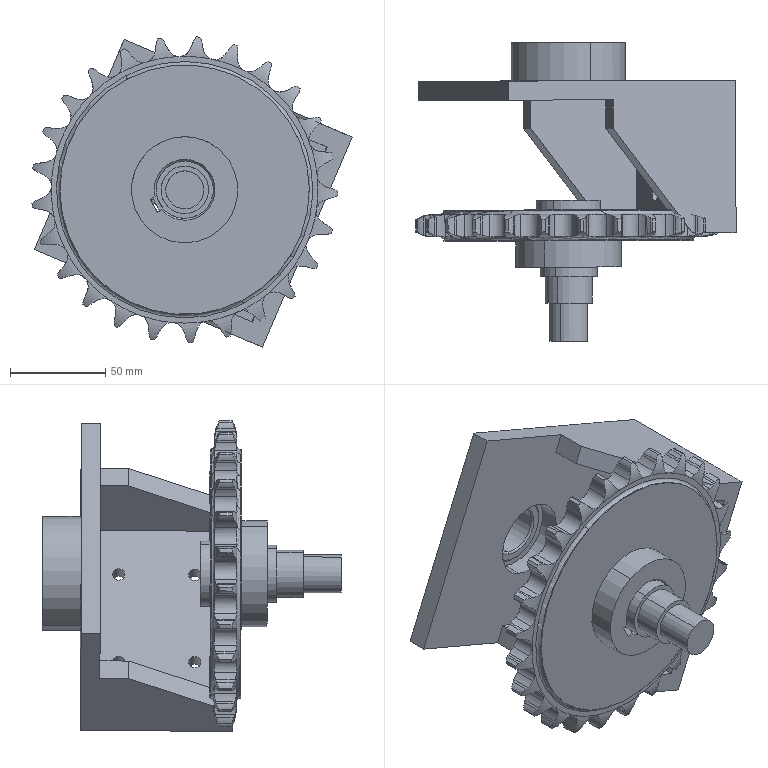Part | NX | features BREP 6 | 6 solids | 460 faces | box 168.151 x 156.922 x 162.976 mm | volume 629639 mm3 | cylinder 217 | plane 105 | torus 70 | sphere 63 | cone 5 | commonest cylinder face diameters 17.202 x53 31.126 x52 12.07 x32 161 x25 6.5 x8 46.4 x8